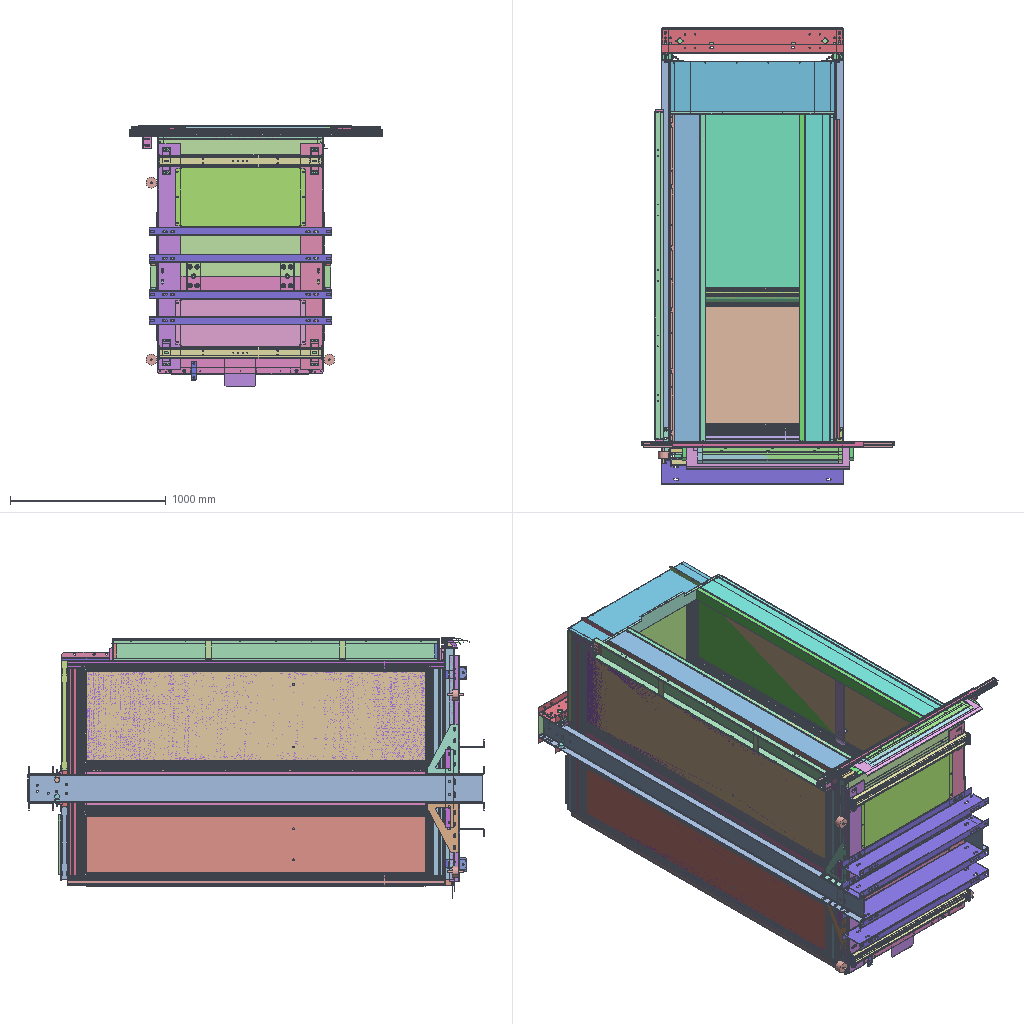Assembly | SolidWorks | 231 different items | 402 placed | box 1620 x 2928 x 1680 mm
Parts list (item | name | quantity | parent item | size | volume | features):
1 | (subassembly) | x1 | in 55 | 1050 x 2251 x 320 mm | 8474214 mm3 | features ReferencePattern 11, MirrorCompFeat 3
2 | (subassembly) | x1 | in 1 | 36 x 2216 x 253 mm | 1745634 mm3 | features ReferencePattern 7, MirrorCompFeat 2
3 | (subassembly) | x1 | in 1 | 36 x 2216 x 253 mm | 1444995 mm3 | features ReferencePattern 8, MirrorCompFeat 3
4 | (subassembly) | x1 | in 49 | 1154 x 89.5 x 1445 mm | 6635667 mm3 | features ReferencePattern 8, MirrorCompFeat 5
5 | (subassembly) | x1 | in 4 | 1050 x 1445 x 59.5 mm | 4576109 mm3 | features ReferencePattern 5, MirrorCompFeat 4, LocalLPattern 1
6 | (subassembly) | x1 | in 7 | 1050 x 70 x 1610 mm | 8250667 mm3 | features ReferencePattern 32, LocalLPattern 5, MirrorCompFeat 5
7 | (subassembly) | x1 | in 49 | 1050 x 70 x 1610 mm | 8250667 mm3 | -
8 | (subassembly) | x1 | in 49 | 1080 x 70 x 1565 mm | 11988496 mm3 | -
9 | (subassembly) | x1 | in 8 | 1080 x 70 x 1565 mm | 10438917 mm3 | features ReferencePattern 25, MirrorCompFeat 7, LocalLPattern 2
10 | (subassembly) | x1 | in 49 | 1050 x 339.8 x 110 mm | 1233242 mm3 | -
11 | (subassembly) | x1 | in 22 | 1170 x 2928 x 820 mm | 20192418 mm3 | features ReferencePattern 8, MirrorCompFeat 7
12 | (subassembly) | x1 | in 10 | 1050 x 339.5 x 110 mm | 828288 mm3 | features MirrorCompFeat 2, ReferencePattern 2
13 | (subassembly) | x1 | in 14 | 225 x 2116 x 80 mm | 1110197 mm3 | features MirrorCompFeat 1, ReferencePattern 1
14 | (subassembly) | x1 | in 49 | 226 x 2116 x 80 mm | 2102242 mm3 | features InContextFeatHolder 1, MirrorCompFeat 1, ReferencePattern 1
15 | (subassembly) | x1 | in 16 | 25 x 2116 x 80 mm | 386202 mm3 | features MirrorCompFeat 1, ReferencePattern 1
16 | (subassembly) | x1 | in 49 | 110.7 x 2116 x 80 mm | 1351065 mm3 | -
17 | (subassembly) | x1 | in 4 | 132 x 50 x 101 mm | 90791 mm3 | -
18 | (subassembly) | x1 | in 4 | 132 x 50 x 101 mm | 90791 mm3 | -
19 | (subassembly) | x1 | in 4 | 132 x 50 x 101 mm | 90791 mm3 | -
20 | (subassembly) | x1 | in 4 | 132 x 50 x 101 mm | 90791 mm3 | -
21 | (subassembly) | x1 | in 50 | 1620 x 178.321 x 70 mm | 5020429 mm3 | -
22 | (subassembly) | x1 | - | 1212 x 2928 x 1450 mm | 26486943 mm3 | -
23 | (subassembly) | x1 | in 24 | 1050 x 60 x 37 mm | 345223 mm3 | features ReferencePattern 5, LocalLPattern 1, MirrorCompFeat 1
24 | (subassembly) | x1 | in 21 | 1620 x 122.321 x 40 mm | 788401 mm3 | features InContextFeatHolder 2
25 | (subassembly) | x1 | in 26 | 50 x 70 x 950 mm | 418927 mm3 | features ReferencePattern 3, LocalLPattern 1, MirrorCompFeat 1
26 | (subassembly) | x1 | in 21 | 60 x 178.321 x 1600 mm | 1702820 mm3 | -
27 | (subassembly) | x1 | in 28 | 60 x 70 x 900 mm | 431961 mm3 | features ReferencePattern 2, MirrorCompFeat 1
28 | (subassembly) | x1 | in 21 | 70 x 143.651 x 1230 mm | 1417083 mm3 | -
29 | (subassembly) | x1 | in 30 | 60 x 70 x 900 mm | 432343 mm3 | features ReferencePattern 2, MirrorCompFeat 1
30 | (subassembly) | x1 | in 21 | 1310 x 141.151 x 70 mm | 1112125 mm3 | -
31 | (subassembly) | x1 | in 50 | - | 153624719 mm3 | -
32 | (subassembly) | x1 | in 31 | 940 x 1360 x 75 mm | 28124716 mm3 | -
33 | (subassembly) | x1 | in 22 | 1212 x 129 x 1450 mm | 5699536 mm3 | features ReferencePattern 16, LocalLPattern 4, MirrorCompFeat 2
34 | (subassembly) | x1 | in 32 | 913 x 1333 x 48 mm | 765196 mm3 | -
35 | (subassembly) | x1 | in 31 | 940 x 1360 x 70 mm | 22273883 mm3 | -
36 | (subassembly) | x1 | in 35 | 939 x 1359 x 25.12 mm | 653415 mm3 | -
37 | (subassembly) | x1 | in 35 | 939 x 1359 x 40 mm | 746249 mm3 | -
38 | (subassembly) | x1 | in 31 | 1360 x 940 x 103 mm | 5180100 mm3 | features ReferencePattern 15, MirrorCompFeat 4, LocalLPattern 1
39 | (subassembly) | x1 | in 31 | 940 x 1360 x 70 mm | 23825388 mm3 | -
40 | (subassembly) | x1 | in 39 | 939 x 1359 x 40 mm | 1439587 mm3 | -
41 | (subassembly) | x1 | in 39 | 939 x 1359 x 40 mm | 1511582 mm3 | -
42 | (subassembly) | x1 | in 31 | 940 x 1360 x 80 mm | 6967858 mm3 | -
43 | (subassembly) | x1 | in 42 | 940 x 1360 x 36 mm | 5509055 mm3 | -
44 | (subassembly) | x1 | in 33 | 145 x 60 x 1450 mm | 1682863 mm3 | -
45 | (subassembly) | x1 | in 42 | 940 x 1360 x 44 mm | 1458803 mm3 | -
46 | (subassembly) | x1 | in 31 | 940 x 1360 x 60.087 mm | 4245748 mm3 | -
47 | (subassembly) | x1 | in 46 | 940 x 1360 x 25.087 mm | 1376149 mm3 | -
48 | (subassembly) | x1 | in 38 | 974.6 x 557 x 34 mm | 203907 mm3 | -
49 | (subassembly) | x1 | in 50 | - | 247371148 mm3 | -
50 | (subassembly) | x1 | - | - | - | features ReferencePattern 2, MirrorCompFeat 1
51 | (subassembly) | x1 | in 52 | 58 x 2100 x 140 mm | 731344 mm3 | features MirrorCompFeat 2, ReferencePattern 2
52 | (subassembly) | x1 | in 50 | 58 x 2132 x 140 mm | 854542 mm3 | -
53 | (subassembly) | x1 | in 33 | 145 x 60 x 1450 mm | 1682863 mm3 | -
54 | (subassembly) | x2 | in 55 | 56.572 x 22.358 x 2390 mm | 591756 mm3 | -
55 | (subassembly) | x1 | in 49 | - | 215809773 mm3 | features ReferencePattern 10, MirrorCompFeat 5
56 | - | x4 | in 33 | 85 x 50 x 6 mm | 24539 mm3 | features Extrusion 1
57 | - | x12 | in 55 | 104 x 104 x 17 mm | 9651 mm3 | features ICE 3, FlatPattern 1, SMBaseFlange 1, SheetMetal 1
58 | - | x4 | in 1 | 240 x 85 x 17 mm | 19751 mm3 | features ICE 3, FlatPattern 1, MirrorPattern 1, SMBaseFlange 1, SheetMetal 1
59 | - | x1 | in 17 | 131 x 50 x 101 mm | 48396 mm3 | features ICE 6, EdgeFlange 1, Fillet 1, FlatPattern 1, SMBaseFlange 1, SheetMetal 1
60 | - | x1 | in 4 | 30 x 2 x 120 mm | 6643 mm3 | features Fillet 1, FlatPattern 1, ICE 1, SMBaseFlange 1, SheetMetal 1
61 | - | x2 | in 17 | 38 x 38 x 50 mm | 20238 mm3 | features Chamfer 2, MoveCopyBody 2, Extrusion 1, ICE 1
62 | - | x1 | in 4 | 1050 x 1 x 1406 mm | 1366400 mm3 | features ICE 10, FlatPattern 2, SMBaseFlange 1, SheetMetal 1
63 | - | x2 | in 4 | 703.5 x 34 x 12 mm | 35744 mm3 | features SMBaseFlange 2, Chamfer 1, Cut 1, EdgeFlange 1, FlatPattern 1, ICE 1, MirrorPattern 1, SheetMetal 1
64 | - | x2 | in 4 | 470 x 34 x 12 mm | 23344 mm3 | features SMBaseFlange 2, Chamfer 1, Cut 1, EdgeFlange 1, FlatPattern 1, ICE 1, MirrorPattern 1, SheetMetal 1
65 | - | x1 | in 18 | 131 x 50 x 101 mm | 48396 mm3 | features MirrorStock 1
66 | - | x1 | in 19 | 131 x 50 x 101 mm | 48396 mm3 | features MirrorStock 1
67 | - | x2 | in 18 | 38 x 38 x 50 mm | 20238 mm3 | features MirrorStock 1
68 | - | x2 | in 19 | 38 x 38 x 50 mm | 20238 mm3 | features MirrorStock 1
69 | - | x1 | in 20 | 131 x 50 x 101 mm | 48396 mm3 | features MirrorStock 1
70 | - | x2 | in 20 | 38 x 38 x 50 mm | 20238 mm3 | features MirrorStock 1
71 | - | x1 | in 23 | 37 x 60 x 1050 mm | 331468 mm3 | features Cut 2, ICE 2, FlatPattern 1, SMBaseFlange 1, SheetMetal 1
72 | - | x6 | in 23 | 30.5 x 48 x 2 mm | 2292 mm3 | features Extrusion 1
73 | - | x1 | in 24 | 17 x 118.321 x 1100 mm | 138591 mm3 | features FlatPattern 1, ICE 1, SMBaseFlange 1, SheetMetal 1
74 | - | x1 | in 24 | 40 x 29.5 x 1620 mm | 304588 mm3 | features Emboss 1, Extrusion 1, ICE 1
75 | - | x1 | in 26 | 17 x 138.321 x 1050 mm | 153799 mm3 | features FlatPattern 1, ICE 1, SMBaseFlange 1, SheetMetal 1
76 | - | x1 | in 25 | 50 x 70 x 950 mm | 401871 mm3 | features ICE 3, FlatPattern 1, SMBaseFlange 1, SheetMetal 1
77 | - | x1 | - | 1046 x 260 x 25 mm | 1454749 mm3 | features ICE 6, Fillet 1, FlatPattern 1, SMBaseFlange 1, SheetMetal 1
78 | - | x4 | in 25 | 43.5 x 60 x 2 mm | 4264 mm3 | features Chamfer 1, Extrusion 1
79 | - | x1 | in 26 | 60 x 40 x 1600 mm | 1130094 mm3 | features Emboss 1, Extrusion 1, ICE 1
80 | - | x1 | in 27 | 60 x 70 x 900 mm | 411225 mm3 | features ICE 3, FlatPattern 1, SMBaseFlange 1, SheetMetal 1
81 | - | x4 | in 27 | 53.5 x 60 x 2 mm | 5184 mm3 | features Chamfer 1, Extrusion 1
82 | - | x1 | in 28 | 70 x 35 x 1230 mm | 881214 mm3 | features Cut 1, Extrusion 1, ICE 1
83 | - | x1 | in 28 | 23.5 x 102.651 x 900 mm | 103908 mm3 | features FlatPattern 1, ICE 1, SMBaseFlange 1, SheetMetal 1
84 | - | x2 | in 30 | 23.5 x 102.651 x 900 mm | 103908 mm3 | features FlatPattern 1, ICE 1, SMBaseFlange 1, SheetMetal 1
85 | - | x1 | in 29 | 60 x 70 x 900 mm | 411607 mm3 | features ICE 3, FlatPattern 1, SMBaseFlange 1, SheetMetal 1
86 | - | x4 | in 29 | 53.5 x 60 x 2 mm | 5184 mm3 | features Chamfer 1, Extrusion 1
87 | - | x1 | in 30 | 70 x 29.5 x 1310 mm | 471967 mm3 | features Emboss 1, Extrusion 1, ICE 1
88 | - | x1 | - | 5 x 19 x 247 mm | 22965 mm3 | features 3DProfileFeature 1, Chamfer 1, Extrusion 1
89 | - | x1 | in 31 | 940 x 1360 x 50 mm | 63007025 mm3 | features ICE 2, Extrusion 1
90 | - | x1 | in 34 | 913 x 1333 x 48 mm | 715108 mm3 | features ICE 7, EdgeFlange 2, FlatPattern 1, SMBaseFlange 1, SheetMetal 1
91 | - | x1 | in 34 | 349.001 x 131.5 x 33.5 mm | 50088 mm3 | features EdgeFlange 1, FlatPattern 1, MirrorPattern 1, SMBaseFlange 1, SheetMetal 1
92 | - | x1 | in 32 | 940 x 1360 x 27 mm | 27359520 mm3 | features ICE 1, WeldMemberFeat 1, WeldmentFeature 1
93 | - | x1 | in 36 | 939 x 1359 x 25 mm | 613016 mm3 | features ICE 7, EdgeFlange 2, FlatPattern 1, SMBaseFlange 1, SheetMetal 1
94 | - | x1 | in 36 | 299 x 128.5 x 17 mm | 40399 mm3 | features EdgeFlange 1, FlatPattern 1, MirrorPattern 1, SMBaseFlange 1, SheetMetal 1
95 | - | x1 | in 35 | 940 x 1360 x 30 mm | 20874219 mm3 | features ICE 1, WeldMemberFeat 1, WeldmentFeature 1
96 | - | x1 | in 37 | 939 x 1359 x 40 mm | 703694 mm3 | features ICE 8, EdgeFlange 2, FlatPattern 1, SMBaseFlange 1, SheetMetal 1
97 | - | x1 | in 37 | 299 x 130.5 x 31 mm | 42555 mm3 | features Cut 1, EdgeFlange 1, FlatPattern 1, MirrorPattern 1, SMBaseFlange 1, SheetMetal 1
98 | - | x1 | in 38 | 1360 x 940 x 50 mm | 873442 mm3 | features Cut 4, EdgeFlange 2, FlatPattern 1, ICE 1, SMBaseFlange 1, SheetMetal 1
99 | - | x2 | in 33 | 40 x 1038 x 70 mm | 337187 mm3 | features FlatPattern 1, ICE 1, SMBaseFlange 1, SheetMetal 1
100 | - | x1 | in 38 | 817.222 x 740.222 x 3 mm | 1814778 mm3 | features Extrusion 1
101 | - | x2 | in 38 | 1356 x 46 x 159 mm | 347836 mm3 | features Cut 5, EdgeFlange 4, SMBaseFlange 2, FlatPattern 1, MirrorPattern 1, SheetMetal 1
102 | - | x2 | in 38 | 668 x 74 x 35 mm | 104821 mm3 | features EdgeFlange 2, Cut 1, FlatPattern 1, ICE 1, SMBaseFlange 1, SheetMetal 1
103 | - | x1 | in 38 | 668 x 74 x 35 mm | 99136 mm3 | features Cut 2, EdgeFlange 2, FlatPattern 1, ICE 1, SMBaseFlange 1, SheetMetal 1
104 | - | x1 | in 38 | 302 x 46 x 116 mm | 44658 mm3 | features Cut 1, EdgeFlange 1, FlatPattern 1, MirrorPattern 1, SMBaseFlange 1, SheetMetal 1, UnFold 1
105 | - | x5 | in 38 | 660 x 74 x 10 mm | 58966 mm3 | features ICE 2, MirrorPattern 2, SMBaseFlange 2, EdgeFlange 1, Fillet 1, FlatPattern 1, SheetMetal 1
106 | - | x1 | in 40 | 939 x 1359 x 40 mm | 1396732 mm3 | features ICE 4, EdgeFlange 2, Cut 1, FlatPattern 1, SMBaseFlange 1, SheetMetal 1
107 | - | x1 | in 40 | 299 x 130.5 x 31 mm | 42855 mm3 | features EdgeFlange 1, FlatPattern 1, MirrorPattern 1, SMBaseFlange 1, SheetMetal 1
108 | - | x1 | in 39 | 940 x 1360 x 30 mm | 20874219 mm3 | features ICE 1, WeldMemberFeat 1, WeldmentFeature 1
109 | - | x1 | in 41 | 939 x 1359 x 40 mm | 1469027 mm3 | features ICE 5, EdgeFlange 2, Cut 1, FlatPattern 1, SMBaseFlange 1, SheetMetal 1
110 | - | x1 | - | 30 x 500 x 50 mm | 112732 mm3 | features ICE 2, FlatPattern 1, SMBaseFlange 1, SheetMetal 1
111 | - | x1 | in 41 | 299 x 130.5 x 31 mm | 42555 mm3 | features Cut 1, EdgeFlange 1, FlatPattern 1, MirrorPattern 1, SMBaseFlange 1, SheetMetal 1
112 | - | x1 | in 43 | 940 x 1360 x 1 mm | 1277171 mm3 | features Cut 2, Extrusion 1
113 | - | x1 | in 43 | 935 x 1355 x 3 mm | 3800775 mm3 | features Extrusion 1
114 | - | x1 | in 45 | 137.5 x 33 x 299 mm | 45429 mm3 | features EdgeFlange 1, FlatPattern 1, MirrorPattern 1, SMBaseFlange 1, SheetMetal 1
115 | - | x1 | in 43 | 940 x 1360 x 35 mm | 431109 mm3 | features WeldMemberFeat 1, WeldmentFeature 1
116 | - | x1 | in 45 | 940 x 1360 x 44 mm | 1413374 mm3 | features ICE 4, EdgeFlange 2, Cut 1, FlatPattern 1, SMBaseFlange 1, SheetMetal 1
117 | - | x1 | in 47 | 940 x 1360 x 25 mm | 1313898 mm3 | features ICE 4, EdgeFlange 2, FlatPattern 1, SMBaseFlange 1, SheetMetal 1
118 | - | x1 | in 47 | 150.5 x 17 x 399 mm | 62251 mm3 | features EdgeFlange 1, FlatPattern 1, MirrorPattern 1, SMBaseFlange 1, SheetMetal 1
119 | - | x1 | in 46 | 1360 x 940 x 35 mm | 2869599 mm3 | features Cut 1, ICE 1, WeldMemberFeat 1, WeldmentFeature 1
120 | - | x2 | in 48 | 957.6 x 538.5 x 32 mm | 71721 mm3 | features FlatPattern 1, SMBaseFlange 1, SheetMetal 1
121 | - | x1 | - | 30 x 557 x 50 mm | 125994 mm3 | features ICE 2, FlatPattern 1, SMBaseFlange 1, SheetMetal 1
122 | - | x1 | in 38 | 1100 x 672 x 0.8 mm | 591119 mm3 | features Cut 1, Extrusion 1
123 | - | x1 | in 48 | 974.6 x 557 x 2 mm | 60464 mm3 | features Extrusion 1, Fillet 1
124 | - | x1 | in 38 | 1062 x 630.2 x 10 mm | 334440 mm3 | features Extrusion 1
125 | - | x1 | in 50 | 225 x 80 x 2116 mm | 3306402 mm3 | features Fillet 6, ICE 5, Extrusion 1, MirrorSolid 1
126 | - | x1 | in 50 | 225 x 80 x 2116 mm | 3306402 mm3 | features Fillet 6, ICE 5, Extrusion 1, MirrorSolid 1
127 | - | x2 | in 50 | 404.961 x 55 x 80 mm | 236837 mm3 | features ICE 2, FlatPattern 1, SMBaseFlange 1, SheetMetal 1
128 | - | x2 | in 50 | 604.961 x 55 x 80 mm | 316837 mm3 | features ICE 2, FlatPattern 1, SMBaseFlange 1, SheetMetal 1
129 | - | x1 | in 50 | 70 x 15 x 800 mm | 506179 mm3 | features ICE 14, Fillet 3, Extrusion 1, MirrorSolid 1
130 | - | x1 | in 51 | 58 x 140 x 2100 mm | 680862 mm3 | features ICE 3, FlatPattern 1, MirrorPattern 1, SMBaseFlange 1, SheetMetal 1
131 | - | x2 | in 51 | 125 x 40 x 2 mm | 10000 mm3 | features Extrusion 1
132 | - | x1 | in 44 | 145 x 60 x 1450 mm | 1662951 mm3 | features ICE 4, Cut 1, EdgeFlange 1, FlatPattern 1, SMBaseFlange 1, SheetMetal 1
133 | - | x2 | in 52 | 56 x 80 x 16 mm | 61599 mm3 | features Extrusion 1, ICE 1
134 | - | x1 | in 51 | 55 x 136 x 30 mm | 15241 mm3 | features Cut 4, EdgeFlange 2, FlatPattern 1, SMBaseFlange 1, SheetMetal 1
135 | - | x1 | in 51 | 55 x 136 x 30 mm | 15241 mm3 | features MirrorStock 1
136 | - | x4 | in 33 | 170 x 52 x 38 mm | 231199 mm3 | features ICE 2, Extrusion 1, MirrorPattern 1, RefAxis 1
137 | - | x1 | in 53 | 145 x 60 x 1450 mm | 1662951 mm3 | features MirrorStock 1
138 | - | x1 | in 22 | 830 x 385 x 10 mm | 330695 mm3 | features ICE 3, EdgeFlange 1, Fillet 1, FlatPattern 1, SMBaseFlange 1, SheetMetal 1
139 | - | x1 | in 11 | 320 x 45 x 200 mm | 197310 mm3 | features MirrorStock 1
140 | - | x1 | in 11 | 320 x 45 x 200 mm | 197310 mm3 | features MirrorStock 1
141 | - | x1 | in 11 | 320 x 45 x 200 mm | 197310 mm3 | features MirrorStock 1
142 | - | x1 | in 50 | 12 x 73 x 1050 mm | 382200 mm3 | features Extrusion 1
143 | - | x2 | in 55 | 630 x 2236 x 18 mm | 13957397 mm3 | features ICE 2, Cut 1, WeldMemberFeat 1, WeldmentFeature 1
144 | - | x2 | in 55 | 420 x 2236 x 18 mm | 9270830 mm3 | features ICE 2, Cut 1, WeldMemberFeat 1, WeldmentFeature 1
145 | - | x1 | in 55 | 1350 x 2236 x 18 mm | 30026574 mm3 | features ICE 3, MirrorPattern 1, WeldMemberFeat 1, WeldmentFeature 1
146 | - | x1 | in 55 | 940 x 2236 x 18 mm | 20877924 mm3 | features ICE 2, WeldMemberFeat 1, WeldmentFeature 1
147 | - | x2 | in 54 | 56.572 x 22.358 x 2385 mm | 399812 mm3 | features Extrusion 1
148 | - | x2 | in 54 | 46.782 x 13.535 x 2390 mm | 191944 mm3 | features Extrusion 1
149 | - | x1 | in 22 | 830 x 305 x 10 mm | 264295 mm3 | features ICE 3, Cut 1, EdgeFlange 1, Fillet 1, FlatPattern 1, SMBaseFlange 1, SheetMetal 1
150 | - | x1 | in 55 | 940 x 2236 x 62.186 mm | 20952715 mm3 | features ICE 7, MirrorSolid 1, WeldMemberFeat 1, WeldmentFeature 1
151 | - | x1 | in 55 | 1050 x 2416 x 1445 mm | 13308461 mm3 | features WeldMemberFeat 5, ICE 4, 3DProfileFeature 1, WeldmentFeature 1
152 | - | x4 | in 1 | 25 x 50 x 2216 mm | 690351 mm3 | features Extrusion 1
153 | - | x4 | in 1 | 14.605 x 34.798 x 2216 mm | 360474 mm3 | features Extrusion 1
154 | - | x4 | in 1 | 9.4 x 46.998 x 2216 mm | 250321 mm3 | features Extrusion 1
155 | - | x1 | in 2 | 240 x 2216 x 23 mm | 917548 mm3 | features Chamfer 2, ICE 2, Cut 1, FlatPattern 1, SMBaseFlange 1, SheetMetal 1
156 | - | x1 | in 2 | 235 x 2216 x 33 mm | 782016 mm3 | features ICE 4, Chamfer 2, Fillet 1, FlatPattern 1, SMBaseFlange 1, SheetMetal 1
157 | - | x2 | in 3 | 30 x 30 x 1181 mm | 101588 mm3 | features Cut 1, Fillet 1, FlatPattern 1, SMBaseFlange 1, SheetMetal 1
158 | - | x1 | in 3 | 240 x 2216 x 23 mm | 637651 mm3 | features Chamfer 2, Cut 2, ICE 2, FlatPattern 1, SMBaseFlange 1, SheetMetal 1
159 | - | x1 | in 3 | 235 x 2216 x 33 mm | 558098 mm3 | features ICE 4, Chamfer 2, Cut 1, Fillet 1, FlatPattern 1, SMBaseFlange 1, SheetMetal 1
160 | - | x3 | in 11 | 160 x 50 x 1170 mm | 1413772 mm3 | features ICE 4, FlatPattern 1, SMBaseFlange 1, SheetMetal 1
161 | - | x24 | in 2, 3 | 12 x 12 x 16.74 mm | 900.506 mm3 | features ICE 2, Extrusion 1, MoveCopyBody 1
162 | - | x4 | in 2, 3 | 10 x 30 x 232 mm | 17632 mm3 | features ExtruThin 1
163 | - | x1 | in 55 | 940 x 2236 x 71.386 mm | 44387536 mm3 | features ICE 13, MirrorSolid 3, LPattern 1, WeldMemberFeat 1, WeldmentFeature 1
164 | - | x1 | in 55 | 1350 x 2236 x 18 mm | 30026574 mm3 | features MirrorStock 1
165 | - | x4 | in 4 | 115 x 90 x 15 mm | 51294 mm3 | features ICE 2, FlatPattern 1, SMBaseFlange 1, SheetMetal 1
166 | - | x2 | in 5 | 969 x 38 x 80 mm | 230143 mm3 | features FlatPattern 1, ICE 1, SMBaseFlange 1, SheetMetal 1
167 | - | x2 | in 5 | 48 x 20 x 380 mm | 82510 mm3 | features FlatPattern 1, SMBaseFlange 1, SheetMetal 1
168 | - | x2 | in 5 | 700 x 38 x 80 mm | 166325 mm3 | features FlatPattern 1, ICE 1, SMBaseFlange 1, SheetMetal 1
169 | - | x1 | in 5 | 1050 x 1445 x 39.5 mm | 2316443 mm3 | features Cut 5, ICE 4, EdgeFlange 2, Fillet 1, FlatPattern 1, SMBaseFlange 1, SheetMetal 1
170 | - | x1 | in 5 | 60 x 38 x 1050 mm | 143033 mm3 | features ICE 3, Cut 2, SMBaseFlange 2, Chamfer 1, Fillet 1, FlatPattern 1, SheetMetal 1
171 | - | x4 | in 11 | 1170 x 160 x 50 mm | 1417867 mm3 | features ICE 5, FlatPattern 1, SMBaseFlange 1, SheetMetal 1
172 | - | x1 | in 5 | 1402 x 38 x 40 mm | 225923 mm3 | features Cut 4, ICE 2, SMBaseFlange 2, FlatPattern 1, SheetMetal 1
173 | - | x2 | in 5 | 320 x 36 x 40 mm | 59416 mm3 | features Cut 2, EdgeFlange 1, FlatPattern 1, SMBaseFlange 1, SheetMetal 1
174 | - | x2 | in 5 | 969 x 38 x 46 mm | 194985 mm3 | features Cut 1, FlatPattern 1, ICE 1, SMBaseFlange 1, SheetMetal 1
175 | - | x1 | in 5 | 969 x 38 x 46 mm | 194985 mm3 | features Cut 1, FlatPattern 1, ICE 1, SMBaseFlange 1, SheetMetal 1
176 | - | x1 | in 5 | 1402 x 38 x 40 mm | 225923 mm3 | features MirrorStock 1
177 | - | x1 | in 6 | 200 x 200 x 3 mm | 119400 mm3 | features Chamfer 1, Extrusion 1
178 | - | x1 | in 6 | 120 x 30 x 2 mm | 6777 mm3 | features Extrusion 1, Fillet 1, ICE 1
179 | - | x24 | in 6 | 68 x 43 x 3 mm | 6956 mm3 | features Chamfer 1, FlatPattern 1, ICE 1, SMBaseFlange 1, SheetMetal 1
180 | - | x6 | in 6 | 26 x 43 x 3 mm | 3279 mm3 | features Chamfer 1, Extrusion 1
181 | - | x1 | in 6 | 72 x 50 x 1520 mm | 718399 mm3 | features ICE 4, Cut 1, Fillet 1, FlatPattern 1, SMBaseFlange 1, SheetMetal 1
182 | - | x2 | in 11 | 180 x 50 x 2908 mm | 3865801 mm3 | features ICE 3, Fillet 2, FlatPattern 1, SMBaseFlange 1, SheetMetal 1
183 | - | x1 | in 6 | 1525 x 70 x 1050 mm | 5031582 mm3 | features ICE 10, Cut 1, Fillet 1, FlatPattern 1, SMBaseFlange 1, SheetMetal 1
184 | - | x7 | in 6 | 25 x 905 x 50 mm | 170375 mm3 | features FlatPattern 1, ICE 1, SMBaseFlange 1, SheetMetal 1
185 | - | x1 | in 6 | 30 x 50 x 905 mm | 273080 mm3 | features Cut 1, FlatPattern 1, ICE 1, SMBaseFlange 1, SheetMetal 1
186 | - | x1 | in 6 | 72 x 50 x 1520 mm | 718399 mm3 | features MirrorStock 1
187 | - | x1 | in 9 | 120 x 30 x 2 mm | 6777 mm3 | features Extrusion 1, Fillet 1, ICE 1
188 | - | x8 | in 9 | 26 x 53 x 3 mm | 4059 mm3 | features Chamfer 1, FlatPattern 1, SMBaseFlange 1, SheetMetal 1
189 | - | x8 | in 9 | 30 x 53 x 3 mm | 4695 mm3 | features Chamfer 1, FlatPattern 1, SMBaseFlange 1, SheetMetal 1
190 | - | x6 | in 9 | 36 x 55 x 3 mm | 5865 mm3 | features Chamfer 1, Extrusion 1
191 | - | x1 | in 9 | 70 x 62 x 1480 mm | 721616 mm3 | features ICE 10, SMBaseFlange 5, Cut 1, FlatPattern 1, SheetMetal 1
192 | - | x2 | in 9 | 40 x 1040 x 62 mm | 524399 mm3 | features SMBaseFlange 2, Cut 1, Fillet 1, FlatPattern 1, SheetMetal 1
193 | - | x1 | in 11 | 320 x 45 x 200 mm | 197310 mm3 | features ICE 8, Fillet 3, FlatPattern 1, SMBaseFlange 1, SheetMetal 1
194 | - | x4 | in 9 | 25 x 1049 x 62 mm | 312113 mm3 | features SMBaseFlange 2, Cut 1, Fillet 1, FlatPattern 1, ICE 1, SheetMetal 1
195 | - | x1 | in 9 | 1525 x 70 x 1060 mm | 5080133 mm3 | features ICE 10, Cut 1, Fillet 1, FlatPattern 1, SMBaseFlange 1, SheetMetal 1
196 | - | x2 | in 9 | 500 x 49 x 4 mm | 94037 mm3 | features FlatPattern 1, ICE 1, MirrorPattern 1, SMBaseFlange 1, SheetMetal 1
197 | - | x2 | in 9 | 500 x 52 x 10 mm | 250092 mm3 | features FlatPattern 1, ICE 1, MirrorPattern 1, SMBaseFlange 1, SheetMetal 1
198 | - | x1 | in 9 | 40 x 62 x 1060 mm | 421378 mm3 | features ICE 2, Cut 1, Fillet 1, FlatPattern 1, SMBaseFlange 1, SheetMetal 1
199 | - | x2 | in 9 | 62 x 200 x 122 mm | 183661 mm3 | features EdgeFlange 1, FlatPattern 1, ICE 1, SMBaseFlange 1, SheetMetal 1
200 | - | x1 | in 8 | 1060 x 1500 x 1 mm | 1549579 mm3 | features ICE 4, FlatPattern 2, Cut 1, Fillet 1, MirrorPattern 1, SMBaseFlange 1, SheetMetal 1
201 | - | x1 | in 9 | 70 x 62 x 1480 mm | 721616 mm3 | features MirrorStock 1
202 | - | x1 | in 12 | 110 x 339.5 x 1050 mm | 713005 mm3 | features ICE 11, Cut 5, EdgeFlange 5, SMBaseFlange 5, Chamfer 1, FlatPattern 1, LPattern 1, SheetMetal 1
203 | - | x1 | in 12 | 336 x 25 x 76.7 mm | 13934 mm3 | features Cut 2, EdgeFlange 2, FlatPattern 1, ICE 1, LPattern 1, SMBaseFlange 1, SheetMetal 1
204 | - | x1 | in 11 | 1160 x 180 x 105 mm | 1758791 mm3 | features FlatPattern 1, ICE 1, SMBaseFlange 1, SheetMetal 1
205 | - | x1 | in 12 | 338 x 15 x 78.5 mm | 43707 mm3 | features ICE 3, Cut 2, EdgeFlange 2, FlatPattern 1, SMBaseFlange 1, SheetMetal 1
206 | - | x1 | in 10 | 323.5 x 64 x 1050 mm | 404954 mm3 | features ICE 2, FlatPattern 1, SMBaseFlange 1, SheetMetal 1
207 | - | x1 | in 12 | 336 x 25 x 76.7 mm | 13934 mm3 | features MirrorStock 1
208 | - | x1 | in 12 | 338 x 15 x 78.5 mm | 43707 mm3 | features MirrorStock 1
209 | - | x1 | in 13 | 221 x 76 x 25 mm | 27869 mm3 | features Cut 5, EdgeFlange 3, ICE 2, FlatPattern 1, MirrorPattern 1, SMBaseFlange 1, SheetMetal 1
210 | - | x1 | in 13 | 225 x 80 x 2116 mm | 1054460 mm3 | features ICE 6, Cut 4, EdgeFlange 2, MirrorPattern 2, Fillet 1, FlatPattern 1, SMBaseFlange 1, SheetMetal 1
211 | - | x1 | in 14 | 98.4 x 25 x 2051 mm | 236423 mm3 | features ICE 2, EdgeFlange 1, FlatPattern 1, SMBaseFlange 1, SheetMetal 1
212 | - | x1 | in 14 | 35 x 18 x 2056 mm | 150261 mm3 | features FlatPattern 1, ICE 1, MirrorPattern 1, SMBaseFlange 1, SheetMetal 1
213 | - | x1 | in 14 | 184 x 24 x 2116 mm | 436728 mm3 | features ICE 2, FlatPattern 1, SMBaseFlange 1, SheetMetal 1
214 | - | x4 | in 33 | 70 x 70 x 106 mm | 159122 mm3 | features ICE 2, Extrusion 1
215 | - | x1 | in 14 | 80 x 1 x 2116 mm | 168632 mm3 | features FlatPattern 1, ICE 1, MirrorPattern 1, SMBaseFlange 1, SheetMetal 1
216 | - | x1 | in 13 | 221 x 76 x 25 mm | 27869 mm3 | features MirrorStock 1
217 | - | x1 | in 15 | 21 x 76 x 25 mm | 6000 mm3 | features Cut 5, EdgeFlange 3, ICE 2, FlatPattern 1, MirrorPattern 1, SMBaseFlange 1, SheetMetal 1
218 | - | x1 | in 15 | 25 x 80 x 2116 mm | 374202 mm3 | features ICE 7, Cut 3, EdgeFlange 2, MirrorPattern 2, Fillet 1, FlatPattern 1, SMBaseFlange 1, SheetMetal 1
219 | - | x1 | in 16 | 98.4 x 25 x 2051 mm | 236423 mm3 | features Cut 1, EdgeFlange 1, FlatPattern 1, ICE 1, SMBaseFlange 1, SheetMetal 1
220 | - | x1 | in 16 | 35 x 35 x 2056 mm | 202689 mm3 | features FlatPattern 1, ICE 1, MirrorPattern 1, SMBaseFlange 1, SheetMetal 1
221 | - | x1 | in 16 | 17 x 30 x 2056 mm | 161613 mm3 | features Cut 1, EdgeFlange 1, FlatPattern 1, ICE 1, SMBaseFlange 1, SheetMetal 1
222 | - | x1 | in 16 | 60 x 34 x 2116 mm | 195504 mm3 | features ICE 2, FlatPattern 1, SMBaseFlange 1, SheetMetal 1
223 | - | x1 | in 16 | 80 x 1 x 2116 mm | 168632 mm3 | features FlatPattern 1, ICE 1, MirrorPattern 1, SMBaseFlange 1, SheetMetal 1
224 | - | x1 | in 15 | 21 x 76 x 25 mm | 6000 mm3 | features MirrorStock 1
225 | - | x1 | - | 85 x 45 x 6 mm | 22107 mm3 | features Extrusion 1
226 | hex nuts, style 1-grades ab gb | x1 | - | - | - | -
227 | hexagon head bolts--product grade c gb | x1 | - | - | - | -
228 | hexagon nuts grade c gb | x1 | - | - | - | -
229 | hexagon weld nuts gb | x1 | - | - | - | -
230 | plain washers--product grade c gb | x1 | - | - | - | -
231 | plain washers-n series-grade a gb | x1 | - | - | - | -
Mates (type | each side: item.copy, entity, surface, feature), first 410 of 702 lines:
In the top assembly
Coincident | 50.1 plane | 22.1 plane | 2 times
Coincident | 186.1 face plane 26-3844 Car Floor Both Sides Rib_Mirror | 136.1 face plane Boss-Extrude 2
In subassembly 50
Coincident | 50.2 face | 50.2 face
Concentric | 50.2 face | 50.2 face
Coincident | 49.1 plane | 50.2 plane | 3 times
DistanceDim | 151.1 face plane 25 Profile 25 Profile Small Post (Latest)(1) | 71.1 face plane Base-Flange 1
DistanceDim | 74.1 face plane Boss-Extrude 1 | 151.1 face plane 25 Profile 25 Profile Small Post (Latest)(1)
Coincident | 151.1 plane | 21.1 plane
Coincident | 183.1 face plane Base-Flange 1 | 126.1 face plane Mirror 1
Coincident | 183.1 face plane Base-Flange 1 | 125.1 face plane Boss-Extrude 3
Coincident | 151.1 face plane 25 Profile 25 Profile Small Post (Latest)(1) | 125.1 face plane Boss-Extrude 2
Coincident | 151.1 face plane 25 Profile 25 Profile Small Post (Latest)(1) | 129.1 face plane Boss-Extrude 1 | 2 times
Coincident | 151.1 plane | 129.1 plane
Coincident | 74.1 face plane Boss-Extrude 1 | 142.1 face plane Boss-Extrude 1
Coincident | 71.1 face plane Base-Flange 1 | 142.1 face plane Boss-Extrude 1
Coincident | 142.1 plane | 50.2 plane
Coincident | 151.1 face plane 25 Profile 25 Profile Small Post (Latest)(1) | 130.1 face plane Base-Flange 1
Coincident | 151.1 face plane 25 Profile 25 Profile Small Post (Latest)(1) | 126.1 face plane Boss-Extrude 2
Coincident | 151.1 face plane 25 Profile 25 Profile Small Post (Latest)(1) | 126.1 face plane Boss-Extrude 1
Coincident | 151.1 face plane 25 Car GC505&506(1) | 125.1 face plane Boss-Extrude 1
DistanceDim | 89.1 face plane Boss-Extrude 1 | 151.1 face plane 25 Car GC505&506(1) | 2 times
Coincident | 169.1 face plane Base-Flange 1 | 89.1 face plane Boss-Extrude 1
Coincident | 143.1 face plane Boss-Extrude 1 | 128.1 face plane Boss-Extrude 1
Concentric | 143.1 face cylinder Cut-Extrude 1 | 128.1 face cylinder Cut-Extrude 1 | 2 times
Coincident | 144.1 face plane Boss-Extrude 1 | 127.1 face plane Boss-Extrude 1
Concentric | 144.1 face cylinder Cut-Extrude 1 | 127.1 face cylinder Cut-Extrude 1 | 2 times
In subassembly 49
Coincident | 49.2 face | 49.2 face
Concentric | 49.2 face | 49.2 face
Coincident | 55.1 plane | 49.2 plane | 3 times
Coincident | 4.1 plane | 49.2 plane | 2 times
Coincident | 151.2 face plane  D:\xxxxxx\xxxx\xxxx\xxxx\xxxx\xxxxxxxxxx(1) | 169.2 face plane Base-Flange 1
Coincident | 10.1 plane | 49.2 plane
Coincident | 7.1 plane | 49.2 plane | 2 times
Coincident | 151.2 face plane  D:\xxxxxx\xxxx\xxxx\xxxx\xxxx\xxxxxxxxxx(1) | 183.2 face plane Base-Flange 1
Coincident | 183.2 face plane Base-Flange 1 | 216.1 face plane
Coincident | 9.1 plane | 49.2 plane
Coincident | 151.2 face plane 25 Car GC503(1) | 195.1 face plane Base-Flange 1
Coincident | 8.1 plane | 49.2 plane
Coincident | 151.2 face plane 25 Profile 25 Profile Small Post (Latest)(1) | 217.1 face plane Base-Flange 1
Coincident | 151.2 face plane 25 Profile 25 Profile Small Post (Latest)(1) | 202.1 face plane Base-Flange 1
Coincident | 151.2 face plane 25 Profile 25 Profile Small Post (Latest)(1) | 210.1 face plane Base-Flange 1 | 2 times
Coincident | 151.2 face plane 25 Profile 25 Profile Small Post (Latest)(1) | 218.1 face plane Base-Flange 1 | 2 times
Coincident | 202.1 face plane Base-Flange 1 | 218.1 face plane Base-Flange 1
In subassembly 55
Coincident | 55.2 face | 55.2 face
Concentric | 55.2 face | 55.2 face
Coincident | 151.3 plane | 55.2 plane | 3 times
Coincident | 1.1 plane | 55.2 plane | 2 times
Coincident | 151.3 face plane 25 Car GC503(1) | 152.1 face plane Boss-Extrude 1
Width | 57.1 face plane Base-Flange 1 | 57.1 face plane Base-Flange 1 | 151.3 face plane 25 Car GC503(1) | 151.3 face plane 25 Car GC503(1)
Coincident | 151.3 face plane 25 Car GC503(1) | 57.1 face plane Base-Flange 1
Coincident | 151.3 face plane  D:\xxxxxx\xxxx\xxxx\xxxx\xxxx\xxxxxxxxxx(1) | 57.1 face plane Base-Flange 1
Coincident | 151.3 face plane  D:\xxxxxx\xxxx\xxxx\xxxx\xxxx\xxxxxxxxxx(1) | 57.2 face plane Base-Flange 1
Parallel | 57.2 edge | 57.1 face plane Base-Flange 1
Coincident | 57.1 edge | 57.2 face plane Base-Flange 1
Coincident | 151.3 face plane 25 Car GC505&506(1) | 57.2 face plane Base-Flange 1
Coincident | 57.1 face plane Base-Flange 1 | 57.3 face plane Base-Flange 1
Coincident | 151.3 face plane  D:\xxxxxx\xxxx\xxxx\xxxx\xxxx\xxxxxxxxxx(1) | 57.3 face plane Base-Flange 1
Width | 57.3 face plane Base-Flange 1 | 57.3 face plane Base-Flange 1 | 151.3 face plane 25 Car GC503(1) | 151.3 face plane 25 Car GC503(1)
Coincident | 151.3 face plane 25 Car GC505&506(1) | 57.4 face plane Base-Flange 1
Coincident | 151.3 face plane  D:\xxxxxx\xxxx\xxxx\xxxx\xxxx\xxxxxxxxxx(1) | 57.4 face plane Base-Flange 1
Coincident | 57.3 face plane Base-Flange 1 | 57.4 edge
Coincident | 146.1 face plane  D:\xxxxxx\xx\xxxx\xxxx\xxxxxx\xxx\xxxxxxxxx(1) | 150.1 face plane  D:\xxxxxx\xx\xxxx\xxxx\xxxxxx\xxx\xxxxxxxxx(1) | 3 times
Coincident | 146.1 plane | 55.2 plane
Coincident | 151.3 face plane 25 Car GC503(1) | 146.1 face plane  D:\xxxxxx\xx\xxxx\xxxx\xxxxxx\xxx\xxxxxxxxx(1) | 2 times
Coincident | 151.3 face plane 25 Car GC503(1) | 144.2 face plane  D:\xxxxxx\xx\xxxx\xxxx\xxxxxx\xxx\xxxxxxxxx(1) | 2 times
Coincident | 151.3 face plane 25 Car GC503(1) | 145.1 face plane  D:\xxxxxx\xx\xxxx\xxxx\xxxxxx\xxx\xxxxxxxxx(1) | 2 times
Coincident | 151.3 face plane 25 Car GC503(1) | 143.2 face plane  D:\xxxxxx\xx\xxxx\xxxx\xxxxxx\xxx\xxxxxxxxx(1) | 2 times
DistanceDim | 151.3 edge | 144.2 face plane  D:\xxxxxx\xx\xxxx\xxxx\xxxxxx\xxx\xxxxxxxxx(1)
DistanceDim | 151.3 face plane  D:\xxxxxx\xxxx\xxxx\xxxx\xxxx\xxxxxxxxxx(1) | 145.1 face plane  D:\xxxxxx\xx\xxxx\xxxx\xxxxxx\xxx\xxxxxxxxx(1)
Coincident | 151.3 face plane  D:\xxxxxx\xxxx\xxxx\xxxx\xxxx\xxxxxxxxxx(1) | 147.1 face plane Boss-Extrude 1
Width | 147.1 face plane Boss-Extrude 1 | 147.1 face plane Boss-Extrude 1 | 151.3 face plane  D:\xxxxxx\xxxx\xxxx\xxxx\xxxx\xxxxxxxxxx(1) | 151.3 face plane  D:\xxxxxx\xxxx\xxxx\xxxx\xxxx\xxxxxxxxxx(1)
Coincident | 151.3 face plane  D:\xxxxxx\xxxx\xxxx\xxxx\xxxx\xxxxxxxxxx(1) | 148.1 face plane Boss-Extrude 1
DistanceDim | 143.2 face plane  D:\xxxxxx\xx\xxxx\xxxx\xxxxxx\xxx\xxxxxxxxx(1) | 152.1 edge
Coincident | 57.3 face plane Base-Flange 1 | 57.5 face plane Base-Flange 1 | 2 times
Coincident | 151.3 face plane 25 Profile 25 Profile Small Post (Latest)(1) | 57.5 face plane Base-Flange 1
Coincident | 57.5 face plane Base-Flange 1 | 57.6 face plane Base-Flange 1
Coincident | 57.4 face plane Base-Flange 1 | 57.6 face plane Base-Flange 1
Coincident | 57.4 edge | 57.6 face plane Base-Flange 1
Coincident | 146.1 face plane  D:\xxxxxx\xx\xxxx\xxxx\xxxxxx\xxx\xxxxxxxxx(1) | 163.1 face plane  D:\xxxxxx\xx\xxxx\xxxx\xxxxxx\xxx\xxxxxxxxx(1) | 3 times
In subassembly 54
Coincident | 54.1 face | 54.1 face
Concentric | 54.1 face | 54.1 face
Coincident | 147.2 plane | 54.1 plane | 3 times
Coincident | 148.2 plane | 54.1 plane | 3 times
In subassembly 1
Coincident | 1.2 face | 1.2 face
Concentric | 1.2 face | 1.2 face
Parallel | 152.2 face plane Boss-Extrude 1 | 1.2 plane | 2 times
Coincident | 152.2 face plane Boss-Extrude 1 | 153.1 face plane Boss-Extrude 1 | 2 times
Coincident | 152.2 plane | 1.2 plane
Coincident | 153.1 plane | 1.2 plane
DistanceDim | 153.1 face plane Boss-Extrude 1 | 154.1 face plane Boss-Extrude 1
Coincident | 154.1 plane | 1.2 plane
Coincident | 153.1 face plane Boss-Extrude 1 | 154.1 edge
Coincident | 152.2 face plane Boss-Extrude 1 | 1.2 select_type:10 | 2 times
Coincident | 3.1 plane | 1.2 plane | 2 times
Coincident | 158.1 face plane Base-Flange 1 | 152.3 face plane Boss-Extrude 1
Coincident | 152.4 face plane Boss-Extrude 1 | 155.1 face plane Base-Flange 1
Coincident | 58.1 plane | 1.2 plane
DistanceDim | 158.1 face plane Base-Flange 1 | 58.1 face plane Base-Flange 1
DistanceDim | 58.1 face plane Base-Flange 1 | 152.3 face plane Boss-Extrude 1
Coincident | 58.2 plane | 1.2 plane
Coincident | 58.1 face plane Base-Flange 1 | 58.2 face plane Base-Flange 1
DistanceDim | 152.2 face plane Boss-Extrude 1 | 58.2 face plane Base-Flange 1
Coincident | 2.1 plane | 1.2 plane | 2 times
In subassembly 3
Coincident | 3.2 face | 3.2 face
Concentric | 3.2 face | 3.2 face
Coincident | 158.2 plane | 3.2 plane | 2 times
Coincident | 158.2 face plane Base-Flange 1 | 3.2 plane
Coincident | 159.1 plane | 3.2 plane | 2 times
Concentric | 158.2 face cylinder Cut-Extrude 2 | 159.1 face cylinder Cut-Extrude 2
Coincident | 159.1 face plane Base-Flange 1 | 157.1 face plane Base-Flange 1
Coincident | 159.1 plane | 157.1 plane
Coincident | 159.1 face plane Cut-Extrude 5 | 157.1 face plane Base-Flange 1
Coincident | 159.1 face plane Base-Flange 1 | 162.1 face plane Extrude-Thin Wall 1 | 2 times
Coincident | 162.1 plane | 3.2 plane
Concentric | 158.2 face cylinder Cut-Extrude 2 | 161.1 face cylinder Boss-Extrude 3
Coincident | 158.2 face plane Base-Flange 1 | 161.1 face plane Boss-Extrude 2
Concentric | 158.2 face cylinder Cut-Extrude 2 | 161.2 face cylinder Boss-Extrude 2
Coincident | 158.2 face plane Base-Flange 1 | 161.2 face plane Boss-Extrude 2
Concentric | 158.2 face cylinder Cut-Extrude 2 | 161.3 face cylinder Boss-Extrude 2
Coincident | 158.2 face plane Base-Flange 1 | 161.3 face plane Boss-Extrude 2
Concentric | 158.2 face cylinder Cut-Extrude 2 | 161.4 face cylinder Boss-Extrude 2
Coincident | 158.2 face plane Base-Flange 1 | 161.4 face plane Boss-Extrude 2
Concentric | 158.2 face cylinder Cut-Extrude 2 | 161.5 face cylinder Boss-Extrude 2
Coincident | 158.2 face plane Base-Flange 1 | 161.5 face plane Boss-Extrude 2
Concentric | 158.2 face cylinder Cut-Extrude 2 | 161.6 face cylinder Boss-Extrude 2
Coincident | 158.2 face plane Base-Flange 1 | 161.6 face plane Boss-Extrude 2
In subassembly 2
Coincident | 2.2 face | 2.2 face
Concentric | 2.2 face | 2.2 face
Coincident | 155.2 plane | 2.2 plane | 2 times
Coincident | 155.2 face plane Base-Flange 1 | 2.2 plane
Coincident | 156.1 plane | 2.2 plane | 2 times
Concentric | 155.2 face cylinder Cut-Extrude 2 | 156.1 face cylinder Cut-Extrude 2
Coincident | 156.1 face plane Base-Flange 1 | 162.1 face plane Extrude-Thin Wall 1 | 2 times
Coincident | 162.1 plane | 2.2 plane
Concentric | 155.2 face cylinder Cut-Extrude 2 | 161.1 face cylinder Boss-Extrude 3
Coincident | 155.2 face plane Base-Flange 1 | 161.1 face plane Boss-Extrude 2
Concentric | 155.2 face cylinder Cut-Extrude 2 | 161.2 face cylinder Boss-Extrude 2
Coincident | 155.2 face plane Base-Flange 1 | 161.2 face plane Boss-Extrude 2
Concentric | 155.2 face cylinder Cut-Extrude 2 | 161.3 face cylinder Boss-Extrude 2
Coincident | 155.2 face plane Base-Flange 1 | 161.3 face plane Boss-Extrude 2
Concentric | 155.2 face cylinder Cut-Extrude 2 | 161.4 face cylinder Boss-Extrude 2
Coincident | 155.2 face plane Base-Flange 1 | 161.4 face plane Boss-Extrude 2
Concentric | 155.2 face cylinder Cut-Extrude 2 | 161.5 face cylinder Boss-Extrude 2
Coincident | 155.2 face plane Base-Flange 1 | 161.5 face plane Boss-Extrude 2
Concentric | 155.2 face cylinder Cut-Extrude 2 | 161.6 face cylinder Boss-Extrude 2
Coincident | 155.2 face plane Base-Flange 1 | 161.6 face plane Boss-Extrude 2
In subassembly 4
Coincident | 4.2 face | 4.2 face
Concentric | 4.2 face | 4.2 face
Coincident | 5.1 plane | 4.2 plane | 2 times
Coincident | 169.3 face plane Base-Flange 1 | 4.2 plane
Coincident | 173.1 face plane Edge-Flange 1 | 59.1 face plane Base-Flange 1
Coincident | 62.1 plane | 4.2 plane | 2 times
Coincident | 170.1 face plane Base-Flange 1 | 62.1 face plane Base-Flange 1
Coincident | 62.1 face plane Base-Flange 1 | 60.1 face plane Base-Flange 1
Slot | 60.1 face cylinder Cut-Extrude 1 | 170.1 face cylinder Cut-Extrude 5
Parallel | 170.1 face plane Base-Flange 1 | 60.1 face plane Base-Flange 1
DistanceDim | 61.1 face plane Boss-Extrude 1 | 172.1 face plane Base-Flange 1
DistanceDim | 4.2 plane | 61.2 face plane Boss-Extrude 1
Coincident | 172.1 face plane Base-Flange 1 | 64.1 face plane Edge-Flange 1
Coincident | 170.1 face plane Base-Flange 1 | 64.1 face plane Base-Flange 1 | 2 times
Coincident | 172.1 face plane Base-Flange 1 | 63.1 face plane Edge-Flange 1
Coincident | 169.3 face plane Edge-Flange 1 | 63.1 face plane Base-Flange 1 | 2 times
Coincident | 173.2 face plane Edge-Flange 1 | 165.1 face plane Base-Flange 1
DistanceDim | 165.1 face plane Boss-Extrude 1 | 176.1 face plane 26-3844 Car Top Longl Side Beam_Mirror
DistanceDim | 165.1 face plane Boss-Extrude 1 | 165.2 face plane Boss-Extrude 1
In subassembly 18
Coincident | 65.1 face plane 26-3844 Damping Bracket_Mirror | 67.1 face plane 26-3844 Car Anti-Sway Rubber Pad_Mirror
Concentric | 65.1 face cylinder 26-3844 Damping Bracket_Mirror | 67.1 face cylinder 26-3844 Car Anti-Sway Rubber Pad_Mirror
Concentric | 65.1 face cylinder 26-3844 Damping Bracket_Mirror | 67.2 face cylinder 26-3844 Car Anti-Sway Rubber Pad_Mirror
Coincident | 65.1 face plane 26-3844 Damping Bracket_Mirror | 67.2 face plane 26-3844 Car Anti-Sway Rubber Pad_Mirror
In subassembly 20
Coincident | 69.1 face plane Mirror 26-3844 Damping Bracket_Mirror | 70.1 face plane Mirror 26-3844 Car Anti-Sway Rubber Pad_Mirror
Concentric | 69.1 face cylinder Mirror 26-3844 Damping Bracket_Mirror | 70.1 face cylinder Mirror 26-3844 Car Anti-Sway Rubber Pad_Mirror
Concentric | 69.1 face cylinder Mirror 26-3844 Damping Bracket_Mirror | 70.2 face cylinder Mirror 26-3844 Car Anti-Sway Rubber Pad_Mirror
Coincident | 69.1 face plane Mirror 26-3844 Damping Bracket_Mirror | 70.2 face plane Mirror 26-3844 Car Anti-Sway Rubber Pad_Mirror
In subassembly 19
Coincident | 66.1 face plane 26-3844 Damping Bracket_Mirror | 68.1 face plane 26-3844 Car Anti-Sway Rubber Pad_Mirror
Concentric | 66.1 face cylinder 26-3844 Damping Bracket_Mirror | 68.1 face cylinder 26-3844 Car Anti-Sway Rubber Pad_Mirror
Concentric | 66.1 face cylinder 26-3844 Damping Bracket_Mirror | 68.2 face cylinder 26-3844 Car Anti-Sway Rubber Pad_Mirror
Coincident | 66.1 face plane 26-3844 Damping Bracket_Mirror | 68.2 face plane 26-3844 Car Anti-Sway Rubber Pad_Mirror
In subassembly 17
Coincident | 59.2 face plane Edge-Flange 1 | 61.3 face plane Boss-Extrude 1
Concentric | 59.2 face cylinder Cut-Extrude 3 | 61.3 face cylinder Boss-Extrude 2
Concentric | 59.2 face cylinder Cut-Extrude 4 | 61.4 face cylinder Boss-Extrude 2
Coincident | 59.2 face plane Base-Flange 1 | 61.4 face plane Boss-Extrude 1
In subassembly 5
Coincident | 5.2 face | 5.2 face
Concentric | 5.2 face | 5.2 face
Coincident | 169.4 plane | 5.2 plane | 2 times
Coincident | 169.4 face plane Base-Flange 1 | 5.2 plane
Coincident | 169.4 face plane Base-Flange 1 | 170.2 face plane Base-Flange 1 | 2 times
Coincident | 170.2 plane | 5.2 plane
Coincident | 169.4 face plane Base-Flange 1 | 172.2 face plane Base-Flange 1 | 2 times
Coincident | 170.2 face plane Base-Flange 1 | 172.2 face plane Base-Flange 1
Coincident | 169.4 face plane Base-Flange 1 | 174.1 face plane Base-Flange 1
Coincident | 174.1 plane | 5.2 plane
DistanceDim | 174.1 face plane Base-Flange 1 | 169.4 face plane Edge-Flange 1
Coincident | 172.2 face plane Base-Flange 1 | 173.3 face plane Base-Flange 1
Coincident | 172.2 face plane Base-Flange 1 | 173.3 face plane Edge-Flange 1
Coincident | 169.4 face plane Base-Flange 1 | 166.1 face plane Base-Flange 1
Coincident | 166.1 plane | 5.2 plane
Coincident | 169.4 face plane Base-Flange 1 | 168.1 face plane Base-Flange 1
Coincident | 166.1 face plane Base-Flange 1 | 168.1 face plane Base-Flange 1
Coincident | 166.1 plane | 168.1 plane
Coincident | 169.4 face plane Base-Flange 1 | 166.2 face plane Base-Flange 1
Coincident | 168.2 face plane Base-Flange 1 | 166.2 face plane Base-Flange 1
Coincident | 166.2 plane | 5.2 plane
DistanceDim | 166.1 face plane Base-Flange 1 | 170.2 face plane Base-Flange 1
Coincident | 172.2 plane | 173.3 plane
Coincident | 172.2 face plane Base-Flange 1 | 167.1 face plane Base-Flange 1 | 2 times
Coincident | 174.2 face plane Base-Flange 1 | 175.1 face plane Base-Flange 1
Coincident | 169.4 face plane Base-Flange 1 | 175.1 face plane Base-Flange 1
Coincident | 175.1 plane | 5.2 plane
DistanceDim | 170.2 face plane Base-Flange 1 | 167.1 face plane Base-Flange 1
In subassembly 10
Coincident | 10.2 face | 10.2 face
Concentric | 10.2 face | 10.2 face
Coincident | 12.1 plane | 10.2 plane | 3 times
Coincident | 206.1 plane | 10.2 plane
DistanceDim | 206.1 face plane Base-Flange 1 | 207.1 face plane 26-3844 Door Lintel Stiffener_Mirror
DistanceDim | 207.1 face plane 26-3844 Door Lintel Stiffener_Mirror | 206.1 face plane Base-Flange 1
In subassembly 12
Coincident | 12.2 face | 12.2 face
Concentric | 12.2 face | 12.2 face
Coincident | 202.2 plane | 12.2 plane
Coincident | 202.2 face plane Base-Flange 1 | 12.2 plane | 2 times
Coincident | 202.2 face plane Base-Flange 1 | 203.1 face plane Edge-Flange 1
Coincident | 202.2 face plane Base-Flange 1 | 203.1 face plane Edge-Flange 2 | 2 times
Coincident | 202.2 face plane Base-Flange 1 | 205.1 face plane Edge-Flange 1
Coincident | 202.2 face plane Base-Flange 1 | 205.1 face plane Edge-Flange 2
DistanceDim | 205.1 face plane Base-Flange 1 | 202.2 face plane Cut-Extrude 8
In subassembly 14
Coincident | 14.1 face | 14.1 face
Concentric | 14.1 face | 14.1 face
Coincident | 13.1 plane | 14.1 plane | 3 times
Coincident | 213.1 plane | 14.1 plane
DistanceDim | 210.2 face plane Edge-Flange 1 | 213.1 face plane Base-Flange 1
DistanceDim | 210.2 face plane Edge-Flange 2 | 213.1 face plane Base-Flange 1
Coincident | 210.2 face plane Base-Flange 1 | 211.1 face plane Edge-Flange 1
Coincident | 211.1 plane | 14.1 plane | 2 times
Coincident | 210.2 face plane Base-Flange 1 | 212.1 face plane Base-Flange 1
Coincident | 212.1 plane | 14.1 plane
Coincident | 210.2 face plane Base-Flange 1 | assembly face | 2 times
Coincident | 212.1 plane | assembly plane
Coincident | 215.1 plane | 14.1 plane
Coincident | 209.1 plane | 215.1 plane
Coincident | 210.2 face plane Base-Flange 1 | 215.1 face plane Base-Flange 1
In subassembly 13
Coincident | 13.2 face | 13.2 face
Concentric | 13.2 face | 13.2 face
Coincident | 210.3 plane | 13.2 plane | 2 times
Coincident | 210.3 face plane Base-Flange 1 | 13.2 plane
Coincident | 209.2 plane | 13.2 plane | 2 times
Coincident | 210.3 face plane Base-Flange 1 | 209.2 face plane Base-Flange 1
In subassembly 8
Coincident | 8.2 face | 8.2 face
Concentric | 8.2 face | 8.2 face
Coincident | 9.2 plane | 8.2 plane | 3 times
Coincident | 198.1 face plane Base-Flange 1 | 200.1 face plane Base-Flange 1
Coincident | 200.1 plane | 8.2 plane | 2 times
In subassembly 9
Coincident | 9.3 face | 9.3 face
Concentric | 9.3 face | 9.3 face
Coincident | 195.2 plane | 9.3 plane | 3 times
Coincident | 198.2 plane | 9.3 plane
Coincident | 195.2 face plane Base-Flange 1 | 198.2 face plane Base-Flange 1 | 2 times
Coincident | 195.2 face plane Base-Flange 1 | 194.1 face plane Base-Flange 1
Coincident | 194.1 plane | 9.3 plane
Coincident | 198.2 face plane Base-Flange 1 | 190.1 face plane Boss-Extrude 1 | 2 times
Coincident | 198.2 face plane Base-Flange 1 | 190.2 face plane Boss-Extrude 1 | 2 times
DistanceDim | 198.2 face plane Base-Flange 1 | 190.2 face plane Boss-Extrude 1
DistanceDim | 9.3 plane | 190.1 face plane Boss-Extrude 1
Coincident | 195.2 face plane Base-Flange 1 | 191.1 face plane Base-Flange 1 | 2 times
Coincident | 198.2 face plane Base-Flange 1 | 191.1 face plane Base-Flange 1
Coincident | 191.1 face plane Base-Flange 1 | 197.1 face plane Base-Flange 1
Coincident | 197.1 plane | 9.3 plane
Width | 195.2 face plane Base-Flange 1 | 191.1 face plane Base-Flange 1 | 197.1 face plane Base-Flange 1 | 197.1 face plane Base-Flange 1
Coincident | 195.2 face plane Base-Flange 1 | 192.1 face plane Base-Flange 1
Coincident | 192.1 plane | 9.3 plane
DistanceDim | 9.3 plane | 192.1 face plane Base-Flange 1
Coincident | 195.2 face plane Base-Flange 1 | 199.1 face plane Edge-Flange 1
Coincident | 199.1 plane | 9.3 plane
DistanceDim | 199.1 plane | 9.3 plane
Coincident | 195.2 face plane Base-Flange 1 | 194.2 face plane Base-Flange 1
Coincident | 194.2 plane | 9.3 plane
Coincident | 191.1 face plane Base-Flange 1 | 196.1 face plane Base-Flange 1
Coincident | 196.1 plane | 9.3 plane
Width | 191.1 face plane Base-Flange 1 | 191.1 face plane Base-Flange 1 | 196.1 face plane Base-Flange 1 | 196.1 face plane Base-Flange 1
Coincident | 191.1 face plane Base-Flange 1 | 189.1 face plane Base-Flange 1 | 2 times
Coincident | 191.1 face plane Base-Flange 1 | 189.2 face plane Base-Flange 1 | 2 times
Coincident | 191.1 face plane Base-Flange 1 | 189.3 face plane Base-Flange 1 | 2 times
Coincident | 191.1 face plane Base-Flange 1 | 189.4 face plane Base-Flange 1 | 2 times
Coincident | 191.1 face plane Fixed Mounting Hole Cut Off | 189.2 face plane Base-Flange 1
Coincident | 191.1 face plane Fixed Mounting Hole Cut Off | 189.3 face plane Base-Flange 1
Coincident | 191.1 face plane Base-Flange 1 | 188.1 face plane Base-Flange 1 | 2 times
DistanceDim | 9.3 plane | 188.1 face plane Base-Flange 1
Coincident | 191.1 face plane Fixed Mounting Hole Cut Off | 194.2 face plane Base-Flange 1
Coincident | 195.2 face plane Base-Flange 1 | 194.3 face plane Base-Flange 1
Coincident | 194.3 plane | 9.3 plane
Coincident | 195.2 face plane Base-Flange 1 | 194.4 face plane Base-Flange 1
Coincident | 194.4 plane | 9.3 plane
Coincident | 191.1 face plane Middle Front Cutout | 194.3 face plane Base-Flange 1
Coincident | 191.1 face plane Fixed Mounting Hole Cut Off | 194.1 face plane Base-Flange 1
Coincident | 191.1 face plane Middle Rear Cutout | 194.4 face plane Base-Flange 1
Coincident | 191.1 face plane Middle Rear Cutout | 189.1 face plane Base-Flange 1
Coincident | 191.1 face plane Middle Front Cutout | 189.4 face plane Base-Flange 1
Coincident | 198.2 face plane Base-Flange 1 | 187.1 face plane Boss-Extrude 1
Width | 187.1 face plane Boss-Extrude 1 | 187.1 face plane Boss-Extrude 1 | 198.2 face plane Base-Flange 1 | 198.2 face plane Base-Flange 1
DistanceDim | 187.1 plane | 9.3 plane
In subassembly 16
Coincident | 16.1 face | 16.1 face
Concentric | 16.1 face | 16.1 face
Coincident | 15.1 plane | 16.1 plane | 3 times
Coincident | 222.1 plane | 16.1 plane
Coincident | 218.2 face plane Base-Flange 1 | 219.1 face plane Edge-Flange 1
Coincident | 219.1 plane | 16.1 plane | 2 times
Coincident | 218.2 face plane Base-Flange 1 | 220.1 face plane Base-Flange 1
Coincident | 220.1 plane | 16.1 plane
Coincident | 218.2 face plane Base-Flange 1 | 221.1 face plane Base-Flange 1
Coincident | 220.1 plane | 221.1 plane
Coincident | 218.2 face plane Base-Flange 1 | 221.1 face plane Edge-Flange 1
Coincident | 223.1 plane | 16.1 plane
Coincident | 217.2 plane | 223.1 plane
Coincident | 218.2 face plane Base-Flange 1 | 223.1 face plane Base-Flange 1
In subassembly 15
Coincident | 15.2 face | 15.2 face
Concentric | 15.2 face | 15.2 face
Coincident | 218.3 plane | 15.2 plane | 2 times
Coincident | 218.3 face plane Base-Flange 1 | 15.2 plane
Coincident | 217.3 plane | 15.2 plane | 2 times
Coincident | 218.3 face plane Base-Flange 1 | 217.3 face plane Base-Flange 1
In subassembly 7
Coincident | 7.2 face | 7.2 face
Concentric | 7.2 face | 7.2 face
Coincident | 6.1 plane | 7.2 plane | 3 times
In subassembly 6
Coincident | 6.2 face | 6.2 face
Concentric | 6.2 face | 6.2 face
Coincident | 183.3 plane | 6.2 plane | 3 times
Coincident | 185.1 plane | 6.2 plane
Coincident | 183.3 face plane Base-Flange 1 | 185.1 face plane Base-Flange 1 | 2 times
Coincident | 183.3 face plane Base-Flange 1 | 181.1 face plane Base-Flange 1 | 3 times
Coincident | 183.3 face plane Base-Flange 1 | 184.1 face plane Base-Flange 1
Coincident | 184.1 plane | 6.2 plane
DistanceDim | 184.1 face plane Base-Flange 1 | 183.3 face plane Base-Flange 1
Coincident | 185.1 face plane Base-Flange 1 | 180.1 face plane Boss-Extrude 1 | 2 times
Coincident | 185.1 face plane Base-Flange 1 | 180.2 face plane Boss-Extrude 1 | 2 times
DistanceDim | 185.1 face plane Base-Flange 1 | 180.2 face plane Boss-Extrude 1
DistanceDim | 6.2 plane | 180.1 face plane Boss-Extrude 1
Coincident | 181.1 face plane Base-Flange 1 | 179.1 face plane Base-Flange 1
DistanceDim | 181.1 face plane Base-Flange 1 | 179.1 face plane Base-Flange 1
DistanceDim | 179.1 face plane Base-Flange 1 | 183.3 face plane Base-Flange 1
Coincident | 179.1 face plane Base-Flange 1 | 179.2 face plane Base-Flange 1
Coincident | 181.1 face plane Base-Flange 1 | 179.2 face plane Base-Flange 1
DistanceDim | 179.2 face plane Base-Flange 1 | 183.3 face plane Base-Flange 1
Coincident | 181.1 face plane Base-Flange 1 | 179.3 face plane Base-Flange 1
Coincident | 179.1 face plane Base-Flange 1 | 179.3 face plane Base-Flange 1
DistanceDim | 6.2 plane | 179.3 face plane Base-Flange 1
Coincident | 185.1 face plane Base-Flange 1 | 177.1 face plane Boss-Extrude 1
Coincident | 177.1 plane | 6.2 plane
Coincident | 185.1 face plane Base-Flange 1 | 178.1 face plane Boss-Extrude 1
DistanceDim | 178.1 plane | 6.2 plane
Width | 178.1 face plane Boss-Extrude 1 | 178.1 face plane Boss-Extrude 1 | 185.1 face plane Base-Flange 1 | 185.1 face plane Base-Flange 1
Width | 177.1 face plane Boss-Extrude 1 | 177.1 face plane Boss-Extrude 1 | 185.1 face plane Base-Flange 1 | 185.1 face plane Base-Flange 1
In subassembly 52
Coincident | 52.1 face | 52.1 face
Concentric | 52.1 face | 52.1 face
Coincident | 51.1 plane | 52.1 plane | 3 times
Coincident | 130.2 face plane Base-Flange 1 | 133.1 face plane Boss-Extrude 1 | 2 times
Coincident | 135.1 face plane | 133.1 face plane Boss-Extrude 1
Coincident | 134.1 face plane Base-Flange 1 | 133.2 face plane Boss-Extrude 1
Coincident | 130.2 face plane Base-Flange 1 | 133.2 face plane Boss-Extrude 1 | 2 times
In subassembly 51
Coincident | 51.2 face | 51.2 face
Concentric | 51.2 face | 51.2 face
Coincident | 130.3 plane | 51.2 plane | 2 times
Coincident | 130.3 face plane Base-Flange 1 | 51.2 plane
Coincident | 130.3 face plane Base-Flange 1 | 134.2 face plane Base-Flange 1
Coincident | 134.2 plane | 51.2 plane | 2 times
Coincident | 130.3 face plane Base-Flange 1 | 131.1 face plane Boss-Extrude 1
Coincident | 131.1 plane | 51.2 plane
DistanceDim | 130.3 face plane Base-Flange 1 | 131.1 face plane Boss-Extrude 1
In subassembly 21
Coincident | 21.2 face | 21.2 face
Concentric | 21.2 face | 21.2 face
Coincident | 24.1 plane | 21.2 plane | 3 times
Coincident | 71.2 face plane Base-Flange 1 | 80.1 face plane Base-Flange 1
Coincident | 74.2 face plane Boss-Extrude 1 | 82.1 face plane Boss-Extrude 1
Coincident | 28.1 plane | 21.2 plane
Coincident | 26.1 plane | 21.2 plane
Coincident | 71.2 face plane Base-Flange 1 | 76.1 face plane Base-Flange 1
Coincident | 74.2 face plane Boss-Extrude 1 | 79.1 face plane Boss-Extrude 1
Coincident | 71.2 face plane Base-Flange 1 | 85.1 face plane Base-Flange 1
Coincident | 74.2 face plane Boss-Extrude 1 | 87.1 face plane Boss-Extrude 1
In subassembly 28
Coincident | 28.2 face | 28.2 face
Concentric | 28.2 face | 28.2 face
Coincident | 82.2 plane | 28.2 plane | 3 times
Coincident | 83.1 plane | 28.2 plane
Coincident | 82.2 face plane Boss-Extrude 1 | 28.2 plane
Coincident | 82.2 face plane Boss-Extrude 1 | 80.2 face plane Base-Flange 1 | 2 times